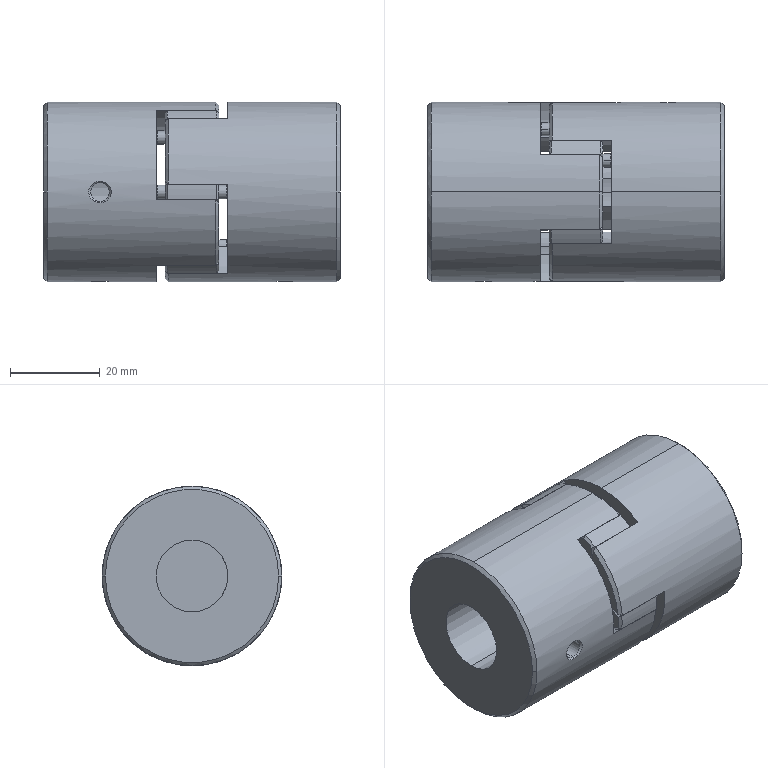Part | SolidWorks | features BaseBody 3 | 3 solids | 188 faces | box 66 x 40 x 40 mm | volume 65274 mm3 | cone 88 | cylinder 80 | plane 20 | commonest cylinder face diameters 23 x35 3 x12 40 x10 4.134 x8 25 x7 16 x4